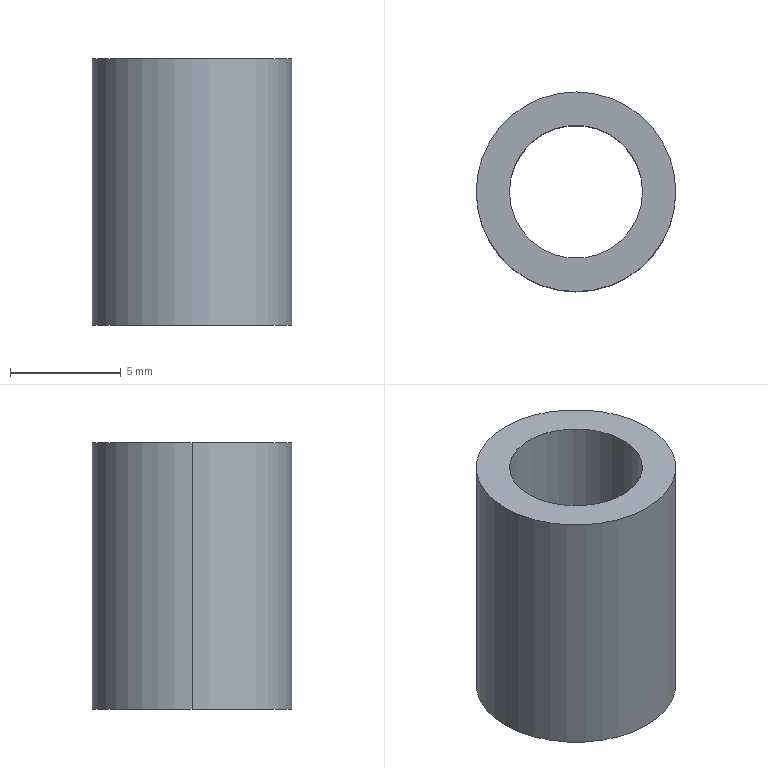Part | STEP file | Ngam kep 10 | 1 solid | 6 faces | box 9 x 9 x 12 mm | volume 424.115 mm3 | cylinder 4 | plane 2 | commonest cylinder face diameters 6 x2 9 x2
STEP:
#1=CARTESIAN_POINT('',(0.,0.,0.));
#2=DIRECTION('',(0.,0.,1.));
#3=DIRECTION('',(1.,0.,0.));
#4=AXIS2_PLACEMENT_3D('',#1,#2,#3);
#5=CARTESIAN_POINT('',(-3.,0.,12.));
#6=VERTEX_POINT('',#5);
#7=CARTESIAN_POINT('',(-3.,0.,0.));
#8=VERTEX_POINT('',#7);
#9=CARTESIAN_POINT('',(-3.,0.,12.));
#10=DIRECTION('',(0.,0.,-1.));
#11=VECTOR('',#10,1.);
#12=LINE('',#9,#11);
#13=CARTESIAN_POINT('',(0.,0.,12.));
#14=DIRECTION('',(0.,0.,-1.));
#15=DIRECTION('',(-1.,0.,0.));
#16=AXIS2_PLACEMENT_3D('',#13,#14,#15);
#17=CYLINDRICAL_SURFACE('',#16,3.);
#18=CARTESIAN_POINT('',(6.283,0.));
#19=DIRECTION('',(0.,1.));
#20=VECTOR('',#19,1.);
#21=LINE('',#18,#20);
#22=(GEOMETRIC_REPRESENTATION_CONTEXT(2)PARAMETRIC_REPRESENTATION_CONTEXT()REPRESENTATION_CONTEXT('',''));
#23=DEFINITIONAL_REPRESENTATION('',(#21),#22);
#24=PCURVE('',#17,#23);
#25=CARTESIAN_POINT('',(0.,0.,12.));
#26=DIRECTION('',(0.,0.,-1.));
#27=DIRECTION('',(-1.,0.,0.));
#28=AXIS2_PLACEMENT_3D('',#25,#26,#27);
#29=CYLINDRICAL_SURFACE('',#28,3.);
#30=CARTESIAN_POINT('',(0.,0.));
#31=DIRECTION('',(0.,1.));
#32=VECTOR('',#31,1.);
#33=LINE('',#30,#32);
#34=(GEOMETRIC_REPRESENTATION_CONTEXT(2)PARAMETRIC_REPRESENTATION_CONTEXT()REPRESENTATION_CONTEXT('',''));
#35=DEFINITIONAL_REPRESENTATION('',(#33),#34);
#36=PCURVE('',#29,#35);
#37=SURFACE_CURVE('',#12,(#24,#36),.PCURVE_S1.);
#38=EDGE_CURVE('',#6,#8,#37,.T.);
#39=ORIENTED_EDGE('',*,*,#38,.T.);
#40=CARTESIAN_POINT('',(3.,0.,0.));
#41=VERTEX_POINT('',#40);
#42=CARTESIAN_POINT('',(0.,0.,0.));
#43=DIRECTION('',(0.,0.,1.));
#44=DIRECTION('',(1.,0.,0.));
#45=AXIS2_PLACEMENT_3D('',#42,#43,#44);
#46=CIRCLE('',#45,3.);
#47=CARTESIAN_POINT('',(9.425,12.));
#48=DIRECTION('',(-1.,0.));
#49=VECTOR('',#48,1.);
#50=LINE('',#47,#49);
#51=(GEOMETRIC_REPRESENTATION_CONTEXT(2)PARAMETRIC_REPRESENTATION_CONTEXT()REPRESENTATION_CONTEXT('',''));
#52=DEFINITIONAL_REPRESENTATION('',(#50),#51);
#53=PCURVE('',#17,#52);
#54=CARTESIAN_POINT('',(0.,0.,0.));
#55=DIRECTION('',(0.,0.,1.));
#56=DIRECTION('',(1.,0.,0.));
#57=AXIS2_PLACEMENT_3D('',#54,#55,#56);
#58=PLANE('',#57);
#59=CARTESIAN_POINT('',(0.,0.));
#60=DIRECTION('',(1.,0.));
#61=AXIS2_PLACEMENT_2D('',#59,#60);
#62=CIRCLE('',#61,3.);
#63=(GEOMETRIC_REPRESENTATION_CONTEXT(2)PARAMETRIC_REPRESENTATION_CONTEXT()REPRESENTATION_CONTEXT('',''));
#64=DEFINITIONAL_REPRESENTATION('',(#62),#63);
#65=PCURVE('',#58,#64);
#66=SURFACE_CURVE('',#46,(#53,#65),.PCURVE_S1.);
#67=EDGE_CURVE('',#8,#41,#66,.T.);
#68=ORIENTED_EDGE('',*,*,#67,.T.);
#69=CARTESIAN_POINT('',(3.,0.,12.));
#70=VERTEX_POINT('',#69);
#71=CARTESIAN_POINT('',(3.,0.,12.));
#72=DIRECTION('',(0.,0.,-1.));
#73=VECTOR('',#72,1.);
#74=LINE('',#71,#73);
#75=CARTESIAN_POINT('',(3.142,0.));
#76=DIRECTION('',(0.,1.));
#77=VECTOR('',#76,1.);
#78=LINE('',#75,#77);
#79=(GEOMETRIC_REPRESENTATION_CONTEXT(2)PARAMETRIC_REPRESENTATION_CONTEXT()REPRESENTATION_CONTEXT('',''));
#80=DEFINITIONAL_REPRESENTATION('',(#78),#79);
#81=PCURVE('',#17,#80);
#82=CARTESIAN_POINT('',(3.142,0.));
#83=DIRECTION('',(0.,1.));
#84=VECTOR('',#83,1.);
#85=LINE('',#82,#84);
#86=(GEOMETRIC_REPRESENTATION_CONTEXT(2)PARAMETRIC_REPRESENTATION_CONTEXT()REPRESENTATION_CONTEXT('',''));
#87=DEFINITIONAL_REPRESENTATION('',(#85),#86);
#88=PCURVE('',#29,#87);
#89=SURFACE_CURVE('',#74,(#81,#88),.PCURVE_S1.);
#90=EDGE_CURVE('',#70,#41,#89,.T.);
#91=ORIENTED_EDGE('',*,*,#90,.F.);
#92=CARTESIAN_POINT('',(0.,0.,12.));
#93=DIRECTION('',(0.,0.,1.));
#94=DIRECTION('',(1.,0.,0.));
#95=AXIS2_PLACEMENT_3D('',#92,#93,#94);
#96=CIRCLE('',#95,3.);
#97=CARTESIAN_POINT('',(9.425,0.));
#98=DIRECTION('',(-1.,0.));
#99=VECTOR('',#98,1.);
#100=LINE('',#97,#99);
#101=(GEOMETRIC_REPRESENTATION_CONTEXT(2)PARAMETRIC_REPRESENTATION_CONTEXT()REPRESENTATION_CONTEXT('',''));
#102=DEFINITIONAL_REPRESENTATION('',(#100),#101);
#103=PCURVE('',#17,#102);
#104=CARTESIAN_POINT('',(0.,0.,12.));
#105=DIRECTION('',(0.,0.,1.));
#106=DIRECTION('',(1.,0.,0.));
#107=AXIS2_PLACEMENT_3D('',#104,#105,#106);
#108=PLANE('',#107);
#109=CARTESIAN_POINT('',(0.,0.));
#110=DIRECTION('',(1.,0.));
#111=AXIS2_PLACEMENT_2D('',#109,#110);
#112=CIRCLE('',#111,3.);
#113=(GEOMETRIC_REPRESENTATION_CONTEXT(2)PARAMETRIC_REPRESENTATION_CONTEXT()REPRESENTATION_CONTEXT('',''));
#114=DEFINITIONAL_REPRESENTATION('',(#112),#113);
#115=PCURVE('',#108,#114);
#116=SURFACE_CURVE('',#96,(#103,#115),.PCURVE_S1.);
#117=EDGE_CURVE('',#6,#70,#116,.T.);
#118=ORIENTED_EDGE('',*,*,#117,.F.);
#119=EDGE_LOOP('',(#39,#68,#91,#118));
#120=FACE_BOUND('',#119,.F.);
#121=ADVANCED_FACE('',(#120),#17,.F.);
#122=CARTESIAN_POINT('',(4.5,0.,12.));
#123=VERTEX_POINT('',#122);
#124=CARTESIAN_POINT('',(-4.5,0.,12.));
#125=VERTEX_POINT('',#124);
#126=CARTESIAN_POINT('',(0.,0.,12.));
#127=DIRECTION('',(0.,0.,1.));
#128=DIRECTION('',(1.,0.,0.));
#129=AXIS2_PLACEMENT_3D('',#126,#127,#128);
#130=CIRCLE('',#129,4.5);
#131=CARTESIAN_POINT('',(0.,0.,12.));
#132=DIRECTION('',(0.,0.,-1.));
#133=DIRECTION('',(-1.,0.,0.));
#134=AXIS2_PLACEMENT_3D('',#131,#132,#133);
#135=CYLINDRICAL_SURFACE('',#134,4.5);
#136=CARTESIAN_POINT('',(3.142,0.));
#137=DIRECTION('',(-1.,0.));
#138=VECTOR('',#137,1.);
#139=LINE('',#136,#138);
#140=(GEOMETRIC_REPRESENTATION_CONTEXT(2)PARAMETRIC_REPRESENTATION_CONTEXT()REPRESENTATION_CONTEXT('',''));
#141=DEFINITIONAL_REPRESENTATION('',(#139),#140);
#142=PCURVE('',#135,#141);
#143=CARTESIAN_POINT('',(0.,0.));
#144=DIRECTION('',(1.,0.));
#145=AXIS2_PLACEMENT_2D('',#143,#144);
#146=CIRCLE('',#145,4.5);
#147=(GEOMETRIC_REPRESENTATION_CONTEXT(2)PARAMETRIC_REPRESENTATION_CONTEXT()REPRESENTATION_CONTEXT('',''));
#148=DEFINITIONAL_REPRESENTATION('',(#146),#147);
#149=PCURVE('',#108,#148);
#150=SURFACE_CURVE('',#130,(#142,#149),.PCURVE_S1.);
#151=EDGE_CURVE('',#123,#125,#150,.T.);
#152=ORIENTED_EDGE('',*,*,#151,.F.);
#153=CARTESIAN_POINT('',(4.5,0.,0.));
#154=VERTEX_POINT('',#153);
#155=CARTESIAN_POINT('',(4.5,0.,12.));
#156=DIRECTION('',(0.,0.,-1.));
#157=VECTOR('',#156,1.);
#158=LINE('',#155,#157);
#159=CARTESIAN_POINT('',(3.142,0.));
#160=DIRECTION('',(0.,1.));
#161=VECTOR('',#160,1.);
#162=LINE('',#159,#161);
#163=(GEOMETRIC_REPRESENTATION_CONTEXT(2)PARAMETRIC_REPRESENTATION_CONTEXT()REPRESENTATION_CONTEXT('',''));
#164=DEFINITIONAL_REPRESENTATION('',(#162),#163);
#165=PCURVE('',#135,#164);
#166=CARTESIAN_POINT('',(0.,0.,12.));
#167=DIRECTION('',(0.,0.,-1.));
#168=DIRECTION('',(-1.,0.,0.));
#169=AXIS2_PLACEMENT_3D('',#166,#167,#168);
#170=CYLINDRICAL_SURFACE('',#169,4.5);
#171=CARTESIAN_POINT('',(3.142,0.));
#172=DIRECTION('',(0.,1.));
#173=VECTOR('',#172,1.);
#174=LINE('',#171,#173);
#175=(GEOMETRIC_REPRESENTATION_CONTEXT(2)PARAMETRIC_REPRESENTATION_CONTEXT()REPRESENTATION_CONTEXT('',''));
#176=DEFINITIONAL_REPRESENTATION('',(#174),#175);
#177=PCURVE('',#170,#176);
#178=SURFACE_CURVE('',#158,(#165,#177),.PCURVE_S1.);
#179=EDGE_CURVE('',#123,#154,#178,.T.);
#180=ORIENTED_EDGE('',*,*,#179,.T.);
#181=CARTESIAN_POINT('',(-4.5,0.,0.));
#182=VERTEX_POINT('',#181);
#183=CARTESIAN_POINT('',(0.,0.,0.));
#184=DIRECTION('',(0.,0.,1.));
#185=DIRECTION('',(1.,0.,0.));
#186=AXIS2_PLACEMENT_3D('',#183,#184,#185);
#187=CIRCLE('',#186,4.5);
#188=CARTESIAN_POINT('',(3.142,12.));
#189=DIRECTION('',(-1.,0.));
#190=VECTOR('',#189,1.);
#191=LINE('',#188,#190);
#192=(GEOMETRIC_REPRESENTATION_CONTEXT(2)PARAMETRIC_REPRESENTATION_CONTEXT()REPRESENTATION_CONTEXT('',''));
#193=DEFINITIONAL_REPRESENTATION('',(#191),#192);
#194=PCURVE('',#135,#193);
#195=CARTESIAN_POINT('',(0.,0.));
#196=DIRECTION('',(1.,0.));
#197=AXIS2_PLACEMENT_2D('',#195,#196);
#198=CIRCLE('',#197,4.5);
#199=(GEOMETRIC_REPRESENTATION_CONTEXT(2)PARAMETRIC_REPRESENTATION_CONTEXT()REPRESENTATION_CONTEXT('',''));
#200=DEFINITIONAL_REPRESENTATION('',(#198),#199);
#201=PCURVE('',#58,#200);
#202=SURFACE_CURVE('',#187,(#194,#201),.PCURVE_S1.);
#203=EDGE_CURVE('',#154,#182,#202,.T.);
#204=ORIENTED_EDGE('',*,*,#203,.T.);
#205=CARTESIAN_POINT('',(-4.5,0.,12.));
#206=DIRECTION('',(0.,0.,-1.));
#207=VECTOR('',#206,1.);
#208=LINE('',#205,#207);
#209=CARTESIAN_POINT('',(0.,0.));
#210=DIRECTION('',(0.,1.));
#211=VECTOR('',#210,1.);
#212=LINE('',#209,#211);
#213=(GEOMETRIC_REPRESENTATION_CONTEXT(2)PARAMETRIC_REPRESENTATION_CONTEXT()REPRESENTATION_CONTEXT('',''));
#214=DEFINITIONAL_REPRESENTATION('',(#212),#213);
#215=PCURVE('',#135,#214);
#216=CARTESIAN_POINT('',(6.283,0.));
#217=DIRECTION('',(0.,1.));
#218=VECTOR('',#217,1.);
#219=LINE('',#216,#218);
#220=(GEOMETRIC_REPRESENTATION_CONTEXT(2)PARAMETRIC_REPRESENTATION_CONTEXT()REPRESENTATION_CONTEXT('',''));
#221=DEFINITIONAL_REPRESENTATION('',(#219),#220);
#222=PCURVE('',#170,#221);
#223=SURFACE_CURVE('',#208,(#215,#222),.PCURVE_S1.);
#224=EDGE_CURVE('',#125,#182,#223,.T.);
#225=ORIENTED_EDGE('',*,*,#224,.F.);
#226=EDGE_LOOP('',(#152,#180,#204,#225));
#227=FACE_BOUND('',#226,.T.);
#228=ADVANCED_FACE('',(#227),#135,.T.);
#229=CARTESIAN_POINT('',(0.,0.,12.));
#230=DIRECTION('',(0.,0.,1.));
#231=DIRECTION('',(1.,0.,0.));
#232=AXIS2_PLACEMENT_3D('',#229,#230,#231);
#233=CIRCLE('',#232,4.5);
#234=CARTESIAN_POINT('',(0.,0.));
#235=DIRECTION('',(1.,0.));
#236=AXIS2_PLACEMENT_2D('',#234,#235);
#237=CIRCLE('',#236,4.5);
#238=(GEOMETRIC_REPRESENTATION_CONTEXT(2)PARAMETRIC_REPRESENTATION_CONTEXT()REPRESENTATION_CONTEXT('',''));
#239=DEFINITIONAL_REPRESENTATION('',(#237),#238);
#240=PCURVE('',#108,#239);
#241=CARTESIAN_POINT('',(9.425,0.));
#242=DIRECTION('',(-1.,0.));
#243=VECTOR('',#242,1.);
#244=LINE('',#241,#243);
#245=(GEOMETRIC_REPRESENTATION_CONTEXT(2)PARAMETRIC_REPRESENTATION_CONTEXT()REPRESENTATION_CONTEXT('',''));
#246=DEFINITIONAL_REPRESENTATION('',(#244),#245);
#247=PCURVE('',#170,#246);
#248=SURFACE_CURVE('',#233,(#240,#247),.PCURVE_S1.);
#249=EDGE_CURVE('',#125,#123,#248,.T.);
#250=ORIENTED_EDGE('',*,*,#249,.T.);
#251=ORIENTED_EDGE('',*,*,#151,.T.);
#252=EDGE_LOOP('',(#250,#251));
#253=FACE_BOUND('',#252,.T.);
#254=ORIENTED_EDGE('',*,*,#117,.F.);
#255=CARTESIAN_POINT('',(0.,0.,12.));
#256=DIRECTION('',(0.,0.,1.));
#257=DIRECTION('',(1.,0.,0.));
#258=AXIS2_PLACEMENT_3D('',#255,#256,#257);
#259=CIRCLE('',#258,3.);
#260=CARTESIAN_POINT('',(0.,0.));
#261=DIRECTION('',(1.,0.));
#262=AXIS2_PLACEMENT_2D('',#260,#261);
#263=CIRCLE('',#262,3.);
#264=(GEOMETRIC_REPRESENTATION_CONTEXT(2)PARAMETRIC_REPRESENTATION_CONTEXT()REPRESENTATION_CONTEXT('',''));
#265=DEFINITIONAL_REPRESENTATION('',(#263),#264);
#266=PCURVE('',#108,#265);
#267=CARTESIAN_POINT('',(3.142,0.));
#268=DIRECTION('',(-1.,0.));
#269=VECTOR('',#268,1.);
#270=LINE('',#267,#269);
#271=(GEOMETRIC_REPRESENTATION_CONTEXT(2)PARAMETRIC_REPRESENTATION_CONTEXT()REPRESENTATION_CONTEXT('',''));
#272=DEFINITIONAL_REPRESENTATION('',(#270),#271);
#273=PCURVE('',#29,#272);
#274=SURFACE_CURVE('',#259,(#266,#273),.PCURVE_S1.);
#275=EDGE_CURVE('',#70,#6,#274,.T.);
#276=ORIENTED_EDGE('',*,*,#275,.F.);
#277=EDGE_LOOP('',(#254,#276));
#278=FACE_BOUND('',#277,.T.);
#279=ADVANCED_FACE('',(#253,#278),#108,.T.);
#280=CARTESIAN_POINT('',(0.,0.,0.));
#281=DIRECTION('',(0.,0.,1.));
#282=DIRECTION('',(1.,0.,0.));
#283=AXIS2_PLACEMENT_3D('',#280,#281,#282);
#284=CIRCLE('',#283,4.5);
#285=CARTESIAN_POINT('',(0.,0.));
#286=DIRECTION('',(1.,0.));
#287=AXIS2_PLACEMENT_2D('',#285,#286);
#288=CIRCLE('',#287,4.5);
#289=(GEOMETRIC_REPRESENTATION_CONTEXT(2)PARAMETRIC_REPRESENTATION_CONTEXT()REPRESENTATION_CONTEXT('',''));
#290=DEFINITIONAL_REPRESENTATION('',(#288),#289);
#291=PCURVE('',#58,#290);
#292=CARTESIAN_POINT('',(9.425,12.));
#293=DIRECTION('',(-1.,0.));
#294=VECTOR('',#293,1.);
#295=LINE('',#292,#294);
#296=(GEOMETRIC_REPRESENTATION_CONTEXT(2)PARAMETRIC_REPRESENTATION_CONTEXT()REPRESENTATION_CONTEXT('',''));
#297=DEFINITIONAL_REPRESENTATION('',(#295),#296);
#298=PCURVE('',#170,#297);
#299=SURFACE_CURVE('',#284,(#291,#298),.PCURVE_S1.);
#300=EDGE_CURVE('',#182,#154,#299,.T.);
#301=ORIENTED_EDGE('',*,*,#300,.F.);
#302=ORIENTED_EDGE('',*,*,#203,.F.);
#303=EDGE_LOOP('',(#301,#302));
#304=FACE_BOUND('',#303,.T.);
#305=ORIENTED_EDGE('',*,*,#67,.T.);
#306=CARTESIAN_POINT('',(0.,0.,0.));
#307=DIRECTION('',(0.,0.,1.));
#308=DIRECTION('',(1.,0.,0.));
#309=AXIS2_PLACEMENT_3D('',#306,#307,#308);
#310=CIRCLE('',#309,3.);
#311=CARTESIAN_POINT('',(0.,0.));
#312=DIRECTION('',(1.,0.));
#313=AXIS2_PLACEMENT_2D('',#311,#312);
#314=CIRCLE('',#313,3.);
#315=(GEOMETRIC_REPRESENTATION_CONTEXT(2)PARAMETRIC_REPRESENTATION_CONTEXT()REPRESENTATION_CONTEXT('',''));
#316=DEFINITIONAL_REPRESENTATION('',(#314),#315);
#317=PCURVE('',#58,#316);
#318=CARTESIAN_POINT('',(3.142,12.));
#319=DIRECTION('',(-1.,0.));
#320=VECTOR('',#319,1.);
#321=LINE('',#318,#320);
#322=(GEOMETRIC_REPRESENTATION_CONTEXT(2)PARAMETRIC_REPRESENTATION_CONTEXT()REPRESENTATION_CONTEXT('',''));
#323=DEFINITIONAL_REPRESENTATION('',(#321),#322);
#324=PCURVE('',#29,#323);
#325=SURFACE_CURVE('',#310,(#317,#324),.PCURVE_S1.);
#326=EDGE_CURVE('',#41,#8,#325,.T.);
#327=ORIENTED_EDGE('',*,*,#326,.T.);
#328=EDGE_LOOP('',(#305,#327));
#329=FACE_BOUND('',#328,.T.);
#330=ADVANCED_FACE('',(#304,#329),#58,.F.);
#331=ORIENTED_EDGE('',*,*,#179,.F.);
#332=ORIENTED_EDGE('',*,*,#249,.F.);
#333=ORIENTED_EDGE('',*,*,#224,.T.);
#334=ORIENTED_EDGE('',*,*,#300,.T.);
#335=EDGE_LOOP('',(#331,#332,#333,#334));
#336=FACE_BOUND('',#335,.T.);
#337=ADVANCED_FACE('',(#336),#170,.T.);
#338=ORIENTED_EDGE('',*,*,#326,.T.);
#339=ORIENTED_EDGE('',*,*,#38,.F.);
#340=ORIENTED_EDGE('',*,*,#275,.F.);
#341=ORIENTED_EDGE('',*,*,#90,.T.);
#342=EDGE_LOOP('',(#338,#339,#340,#341));
#343=FACE_BOUND('',#342,.F.);
#344=ADVANCED_FACE('',(#343),#29,.F.);
#345=CLOSED_SHELL('',(#121,#228,#279,#330,#337,#344));
#346=MANIFOLD_SOLID_BREP('',#345);
#347=(LENGTH_UNIT()NAMED_UNIT(*)SI_UNIT(.MILLI.,.METRE.));
#348=UNCERTAINTY_MEASURE_WITH_UNIT(LENGTH_MEASURE(0.0000001),#347,'','');
#349=(NAMED_UNIT(*)PLANE_ANGLE_UNIT()SI_UNIT($,.RADIAN.));
#350=(NAMED_UNIT(*)SI_UNIT($,.STERADIAN.)SOLID_ANGLE_UNIT());
#351=(GEOMETRIC_REPRESENTATION_CONTEXT(3)GLOBAL_UNCERTAINTY_ASSIGNED_CONTEXT((#348))GLOBAL_UNIT_ASSIGNED_CONTEXT((#347,#349,#350))REPRESENTATION_CONTEXT('',''));
#352=ADVANCED_BREP_SHAPE_REPRESENTATION('',(#4,#346),#351);